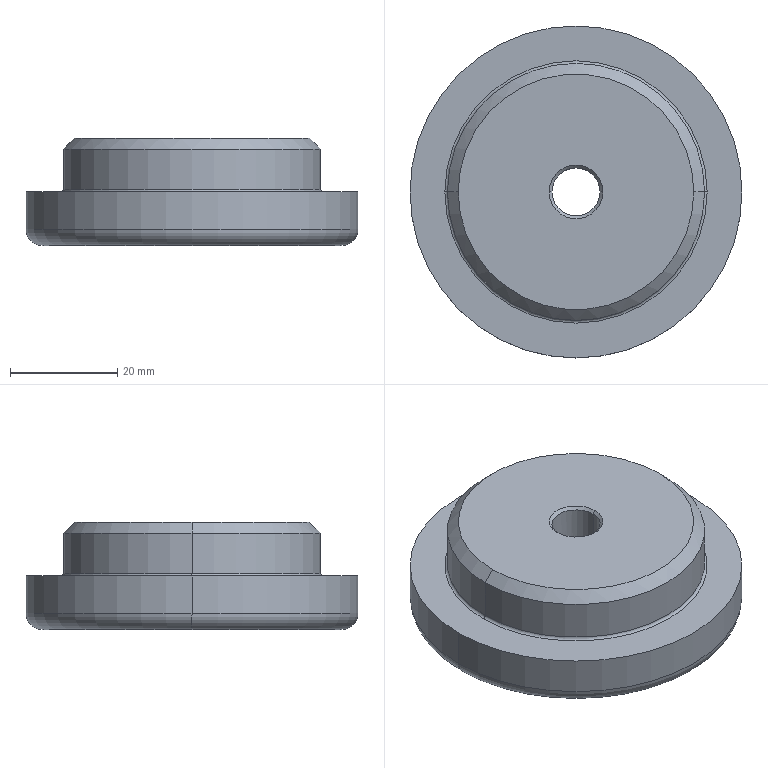Part | SolidWorks | features ICE 3, Fillet 2, 3DProfileFeature 1, Chamfer 1, Extrusion 1, HoleWzd 1 | 1 solid | 37 faces | box 62 x 62 x 20 mm | volume 45800 mm3 | plane 18 | cylinder 11 | torus 4 | cone 4 | commonest cylinder face diameters 6 x5 9 x2 48 x2 62 x2
STEP:
#1=CARTESIAN_POINT('',(-24.,0.,10.5));
#2=VERTEX_POINT('',#1);
#3=CARTESIAN_POINT('',(24.,0.,10.5));
#4=VERTEX_POINT('',#3);
#5=CARTESIAN_POINT('',(0.,0.,10.5));
#6=DIRECTION('',(0.,0.,1.));
#7=DIRECTION('',(1.,0.,0.));
#8=AXIS2_PLACEMENT_3D('',#5,#6,#7);
#9=CIRCLE('',#8,24.);
#10=EDGE_CURVE('',#2,#4,#9,.T.);
#11=ORIENTED_EDGE('',*,*,#10,.F.);
#12=CARTESIAN_POINT('',(-24.5,0.,10.));
#13=VERTEX_POINT('',#12);
#14=CARTESIAN_POINT('',(-24.5,0.,10.5));
#15=DIRECTION('',(0.,1.,0.));
#16=DIRECTION('',(-1.,0.,0.));
#17=AXIS2_PLACEMENT_3D('',#14,#15,#16);
#18=CIRCLE('',#17,0.5);
#19=EDGE_CURVE('',#2,#13,#18,.T.);
#20=ORIENTED_EDGE('',*,*,#19,.T.);
#21=CARTESIAN_POINT('',(24.5,0.,10.));
#22=VERTEX_POINT('',#21);
#23=CARTESIAN_POINT('',(0.,0.,10.));
#24=DIRECTION('',(0.,0.,-1.));
#25=DIRECTION('',(1.,0.,0.));
#26=AXIS2_PLACEMENT_3D('',#23,#24,#25);
#27=CIRCLE('',#26,24.5);
#28=EDGE_CURVE('',#22,#13,#27,.T.);
#29=ORIENTED_EDGE('',*,*,#28,.F.);
#30=CARTESIAN_POINT('',(24.5,0.,10.5));
#31=DIRECTION('',(0.,-1.,0.));
#32=DIRECTION('',(0.,0.,-1.));
#33=AXIS2_PLACEMENT_3D('',#30,#31,#32);
#34=CIRCLE('',#33,0.5);
#35=EDGE_CURVE('',#4,#22,#34,.T.);
#36=ORIENTED_EDGE('',*,*,#35,.F.);
#37=EDGE_LOOP('',(#11,#20,#29,#36));
#38=FACE_OUTER_BOUND('',#37,.T.);
#39=CARTESIAN_POINT('',(0.,0.,10.5));
#40=DIRECTION('',(0.,0.,1.));
#41=DIRECTION('',(1.,0.,0.));
#42=AXIS2_PLACEMENT_3D('',#39,#40,#41);
#43=TOROIDAL_SURFACE('',#42,24.5,0.5);
#44=ADVANCED_FACE('',(#38),#43,.F.);
#45=CARTESIAN_POINT('',(-28.,0.,1.));
#46=VERTEX_POINT('',#45);
#47=CARTESIAN_POINT('',(-25.,3.,1.));
#48=VERTEX_POINT('',#47);
#49=CARTESIAN_POINT('',(-25.,0.,1.));
#50=DIRECTION('',(0.,0.,-1.));
#51=DIRECTION('',(-1.,0.,0.));
#52=AXIS2_PLACEMENT_3D('',#49,#50,#51);
#53=CIRCLE('',#52,3.);
#54=EDGE_CURVE('',#46,#48,#53,.T.);
#55=ORIENTED_EDGE('',*,*,#54,.F.);
#56=CARTESIAN_POINT('',(-28.,0.,0.));
#57=VERTEX_POINT('',#56);
#58=CARTESIAN_POINT('',(-28.,0.,1.));
#59=DIRECTION('',(0.,0.,-1.));
#60=VECTOR('',#59,1000.);
#61=LINE('',#58,#60);
#62=EDGE_CURVE('',#46,#57,#61,.T.);
#63=ORIENTED_EDGE('',*,*,#62,.T.);
#64=CARTESIAN_POINT('',(-25.,3.,0.));
#65=VERTEX_POINT('',#64);
#66=CARTESIAN_POINT('',(-25.,0.,0.));
#67=DIRECTION('',(0.,0.,-1.));
#68=DIRECTION('',(-1.,0.,0.));
#69=AXIS2_PLACEMENT_3D('',#66,#67,#68);
#70=CIRCLE('',#69,3.);
#71=EDGE_CURVE('',#57,#65,#70,.T.);
#72=ORIENTED_EDGE('',*,*,#71,.T.);
#73=CARTESIAN_POINT('',(-25.,3.,1.));
#74=DIRECTION('',(0.,0.,-1.));
#75=VECTOR('',#74,1000.);
#76=LINE('',#73,#75);
#77=EDGE_CURVE('',#48,#65,#76,.T.);
#78=ORIENTED_EDGE('',*,*,#77,.F.);
#79=EDGE_LOOP('',(#55,#63,#72,#78));
#80=FACE_OUTER_BOUND('',#79,.T.);
#81=CARTESIAN_POINT('',(-25.,0.,1.));
#82=DIRECTION('',(0.,0.,-1.));
#83=DIRECTION('',(-1.,0.,0.));
#84=AXIS2_PLACEMENT_3D('',#81,#82,#83);
#85=CYLINDRICAL_SURFACE('',#84,3.);
#86=ADVANCED_FACE('',(#80),#85,.F.);
#87=CARTESIAN_POINT('',(-4.5,0.,19.475));
#88=VERTEX_POINT('',#87);
#89=CARTESIAN_POINT('',(4.5,0.,19.475));
#90=VERTEX_POINT('',#89);
#91=CARTESIAN_POINT('',(0.,0.,19.475));
#92=DIRECTION('',(0.,0.,1.));
#93=DIRECTION('',(1.,0.,0.));
#94=AXIS2_PLACEMENT_3D('',#91,#92,#93);
#95=CIRCLE('',#94,4.5);
#96=EDGE_CURVE('',#88,#90,#95,.T.);
#97=ORIENTED_EDGE('',*,*,#96,.F.);
#98=CARTESIAN_POINT('',(-5.025,0.,20.));
#99=VERTEX_POINT('',#98);
#100=CARTESIAN_POINT('',(-5.025,0.,20.));
#101=DIRECTION('',(-0.7071,0.,0.7071));
#102=VECTOR('',#101,1000.);
#103=LINE('',#100,#102);
#104=EDGE_CURVE('',#88,#99,#103,.T.);
#105=ORIENTED_EDGE('',*,*,#104,.T.);
#106=CARTESIAN_POINT('',(5.025,0.,20.));
#107=VERTEX_POINT('',#106);
#108=CARTESIAN_POINT('',(0.,0.,20.));
#109=DIRECTION('',(0.,0.,1.));
#110=DIRECTION('',(1.,0.,0.));
#111=AXIS2_PLACEMENT_3D('',#108,#109,#110);
#112=CIRCLE('',#111,5.025);
#113=EDGE_CURVE('',#99,#107,#112,.T.);
#114=ORIENTED_EDGE('',*,*,#113,.T.);
#115=CARTESIAN_POINT('',(5.025,0.,20.));
#116=DIRECTION('',(0.7071,0.,0.7071));
#117=VECTOR('',#116,1000.);
#118=LINE('',#115,#117);
#119=EDGE_CURVE('',#90,#107,#118,.T.);
#120=ORIENTED_EDGE('',*,*,#119,.F.);
#121=EDGE_LOOP('',(#97,#105,#114,#120));
#122=FACE_OUTER_BOUND('',#121,.T.);
#123=CARTESIAN_POINT('',(0.,0.,20.));
#124=DIRECTION('',(0.,0.,1.));
#125=DIRECTION('',(1.,0.,0.));
#126=AXIS2_PLACEMENT_3D('',#123,#124,#125);
#127=CONICAL_SURFACE('',#126,5.025,0.7854);
#128=ADVANCED_FACE('',(#122),#127,.F.);
#129=CARTESIAN_POINT('',(-4.5,0.,1.));
#130=VERTEX_POINT('',#129);
#131=CARTESIAN_POINT('',(-3.354,-3.,1.));
#132=VERTEX_POINT('',#131);
#133=CARTESIAN_POINT('',(0.,0.,1.));
#134=DIRECTION('',(0.,0.,1.));
#135=DIRECTION('',(-1.,0.,0.));
#136=AXIS2_PLACEMENT_3D('',#133,#134,#135);
#137=CIRCLE('',#136,4.5);
#138=EDGE_CURVE('',#130,#132,#137,.T.);
#139=ORIENTED_EDGE('',*,*,#138,.F.);
#140=CARTESIAN_POINT('',(-4.5,0.,20.));
#141=DIRECTION('',(0.,0.,1.));
#142=VECTOR('',#141,1000.);
#143=LINE('',#140,#142);
#144=EDGE_CURVE('',#130,#88,#143,.T.);
#145=ORIENTED_EDGE('',*,*,#144,.T.);
#146=ORIENTED_EDGE('',*,*,#96,.T.);
#147=CARTESIAN_POINT('',(4.5,0.,1.));
#148=VERTEX_POINT('',#147);
#149=CARTESIAN_POINT('',(4.5,0.,20.));
#150=DIRECTION('',(0.,0.,1.));
#151=VECTOR('',#150,1000.);
#152=LINE('',#149,#151);
#153=EDGE_CURVE('',#148,#90,#152,.T.);
#154=ORIENTED_EDGE('',*,*,#153,.F.);
#155=CARTESIAN_POINT('',(3.354,-3.,1.));
#156=VERTEX_POINT('',#155);
#157=CARTESIAN_POINT('',(0.,0.,1.));
#158=DIRECTION('',(0.,0.,1.));
#159=DIRECTION('',(-1.,0.,0.));
#160=AXIS2_PLACEMENT_3D('',#157,#158,#159);
#161=CIRCLE('',#160,4.5);
#162=EDGE_CURVE('',#156,#148,#161,.T.);
#163=ORIENTED_EDGE('',*,*,#162,.F.);
#164=CARTESIAN_POINT('',(3.354,-3.,0.));
#165=VERTEX_POINT('',#164);
#166=CARTESIAN_POINT('',(3.354,-3.,20.));
#167=DIRECTION('',(0.,0.,-1.));
#168=VECTOR('',#167,1000.);
#169=LINE('',#166,#168);
#170=EDGE_CURVE('',#156,#165,#169,.T.);
#171=ORIENTED_EDGE('',*,*,#170,.T.);
#172=CARTESIAN_POINT('',(3.,-3.354,0.));
#173=VERTEX_POINT('',#172);
#174=CARTESIAN_POINT('',(0.,0.,0.));
#175=DIRECTION('',(0.,0.,1.));
#176=DIRECTION('',(1.,0.,0.));
#177=AXIS2_PLACEMENT_3D('',#174,#175,#176);
#178=CIRCLE('',#177,4.5);
#179=EDGE_CURVE('',#173,#165,#178,.T.);
#180=ORIENTED_EDGE('',*,*,#179,.F.);
#181=CARTESIAN_POINT('',(3.,-3.354,1.));
#182=VERTEX_POINT('',#181);
#183=CARTESIAN_POINT('',(3.,-3.354,20.));
#184=DIRECTION('',(0.,0.,1.));
#185=VECTOR('',#184,1000.);
#186=LINE('',#183,#185);
#187=EDGE_CURVE('',#173,#182,#186,.T.);
#188=ORIENTED_EDGE('',*,*,#187,.T.);
#189=CARTESIAN_POINT('',(-3.,-3.354,1.));
#190=VERTEX_POINT('',#189);
#191=CARTESIAN_POINT('',(0.,0.,1.));
#192=DIRECTION('',(0.,0.,1.));
#193=DIRECTION('',(-1.,0.,0.));
#194=AXIS2_PLACEMENT_3D('',#191,#192,#193);
#195=CIRCLE('',#194,4.5);
#196=EDGE_CURVE('',#190,#182,#195,.T.);
#197=ORIENTED_EDGE('',*,*,#196,.F.);
#198=CARTESIAN_POINT('',(-3.,-3.354,0.));
#199=VERTEX_POINT('',#198);
#200=CARTESIAN_POINT('',(-3.,-3.354,20.));
#201=DIRECTION('',(0.,0.,-1.));
#202=VECTOR('',#201,1000.);
#203=LINE('',#200,#202);
#204=EDGE_CURVE('',#190,#199,#203,.T.);
#205=ORIENTED_EDGE('',*,*,#204,.T.);
#206=CARTESIAN_POINT('',(-3.354,-3.,0.));
#207=VERTEX_POINT('',#206);
#208=CARTESIAN_POINT('',(0.,0.,0.));
#209=DIRECTION('',(0.,0.,1.));
#210=DIRECTION('',(1.,0.,0.));
#211=AXIS2_PLACEMENT_3D('',#208,#209,#210);
#212=CIRCLE('',#211,4.5);
#213=EDGE_CURVE('',#207,#199,#212,.T.);
#214=ORIENTED_EDGE('',*,*,#213,.F.);
#215=CARTESIAN_POINT('',(-3.354,-3.,20.));
#216=DIRECTION('',(0.,0.,1.));
#217=VECTOR('',#216,1000.);
#218=LINE('',#215,#217);
#219=EDGE_CURVE('',#207,#132,#218,.T.);
#220=ORIENTED_EDGE('',*,*,#219,.T.);
#221=EDGE_LOOP('',(#139,#145,#146,#154,#163,#171,#180,#188,#197,#205,#214,#220));
#222=FACE_OUTER_BOUND('',#221,.T.);
#223=CARTESIAN_POINT('',(0.,0.,20.));
#224=DIRECTION('',(0.,0.,1.));
#225=DIRECTION('',(1.,0.,0.));
#226=AXIS2_PLACEMENT_3D('',#223,#224,#225);
#227=CYLINDRICAL_SURFACE('',#226,4.5);
#228=ADVANCED_FACE('',(#222),#227,.F.);
#229=CARTESIAN_POINT('',(0.,28.,0.));
#230=VERTEX_POINT('',#229);
#231=CARTESIAN_POINT('',(0.,0.,0.));
#232=DIRECTION('',(0.,0.,-1.));
#233=DIRECTION('',(1.,0.,0.));
#234=AXIS2_PLACEMENT_3D('',#231,#232,#233);
#235=CIRCLE('',#234,28.);
#236=EDGE_CURVE('',#57,#230,#235,.T.);
#237=ORIENTED_EDGE('',*,*,#236,.F.);
#238=CARTESIAN_POINT('',(-31.,0.,3.));
#239=VERTEX_POINT('',#238);
#240=CARTESIAN_POINT('',(-28.,0.,3.));
#241=DIRECTION('',(0.,1.,0.));
#242=DIRECTION('',(-1.,0.,0.));
#243=AXIS2_PLACEMENT_3D('',#240,#241,#242);
#244=CIRCLE('',#243,3.);
#245=EDGE_CURVE('',#57,#239,#244,.T.);
#246=ORIENTED_EDGE('',*,*,#245,.T.);
#247=CARTESIAN_POINT('',(31.,0.,3.));
#248=VERTEX_POINT('',#247);
#249=CARTESIAN_POINT('',(0.,0.,3.));
#250=DIRECTION('',(0.,0.,1.));
#251=DIRECTION('',(1.,0.,0.));
#252=AXIS2_PLACEMENT_3D('',#249,#250,#251);
#253=CIRCLE('',#252,31.);
#254=EDGE_CURVE('',#248,#239,#253,.T.);
#255=ORIENTED_EDGE('',*,*,#254,.F.);
#256=CARTESIAN_POINT('',(28.,0.,0.));
#257=VERTEX_POINT('',#256);
#258=CARTESIAN_POINT('',(28.,0.,3.));
#259=DIRECTION('',(0.,-1.,0.));
#260=DIRECTION('',(0.,0.,-1.));
#261=AXIS2_PLACEMENT_3D('',#258,#259,#260);
#262=CIRCLE('',#261,3.);
#263=EDGE_CURVE('',#257,#248,#262,.T.);
#264=ORIENTED_EDGE('',*,*,#263,.F.);
#265=CARTESIAN_POINT('',(0.,0.,0.));
#266=DIRECTION('',(0.,0.,-1.));
#267=DIRECTION('',(1.,0.,0.));
#268=AXIS2_PLACEMENT_3D('',#265,#266,#267);
#269=CIRCLE('',#268,28.);
#270=EDGE_CURVE('',#230,#257,#269,.T.);
#271=ORIENTED_EDGE('',*,*,#270,.F.);
#272=EDGE_LOOP('',(#237,#246,#255,#264,#271));
#273=FACE_OUTER_BOUND('',#272,.T.);
#274=CARTESIAN_POINT('',(0.,0.,3.));
#275=DIRECTION('',(0.,0.,1.));
#276=DIRECTION('',(1.,0.,0.));
#277=AXIS2_PLACEMENT_3D('',#274,#275,#276);
#278=TOROIDAL_SURFACE('',#277,28.,3.);
#279=ADVANCED_FACE('',(#273),#278,.T.);
#280=CARTESIAN_POINT('',(22.,0.,20.));
#281=VERTEX_POINT('',#280);
#282=CARTESIAN_POINT('',(-22.,0.,20.));
#283=VERTEX_POINT('',#282);
#284=CARTESIAN_POINT('',(0.,0.,20.));
#285=DIRECTION('',(0.,0.,1.));
#286=DIRECTION('',(1.,0.,0.));
#287=AXIS2_PLACEMENT_3D('',#284,#285,#286);
#288=CIRCLE('',#287,22.);
#289=EDGE_CURVE('',#281,#283,#288,.T.);
#290=ORIENTED_EDGE('',*,*,#289,.F.);
#291=CARTESIAN_POINT('',(24.,0.,18.));
#292=VERTEX_POINT('',#291);
#293=CARTESIAN_POINT('',(22.,0.,20.));
#294=DIRECTION('',(0.7071,0.,-0.7071));
#295=VECTOR('',#294,1000.);
#296=LINE('',#293,#295);
#297=EDGE_CURVE('',#281,#292,#296,.T.);
#298=ORIENTED_EDGE('',*,*,#297,.T.);
#299=CARTESIAN_POINT('',(-24.,0.,18.));
#300=VERTEX_POINT('',#299);
#301=CARTESIAN_POINT('',(0.,0.,18.));
#302=DIRECTION('',(0.,0.,-1.));
#303=DIRECTION('',(1.,0.,0.));
#304=AXIS2_PLACEMENT_3D('',#301,#302,#303);
#305=CIRCLE('',#304,24.);
#306=EDGE_CURVE('',#300,#292,#305,.T.);
#307=ORIENTED_EDGE('',*,*,#306,.F.);
#308=CARTESIAN_POINT('',(-22.,0.,20.));
#309=DIRECTION('',(-0.7071,0.,-0.7071));
#310=VECTOR('',#309,1000.);
#311=LINE('',#308,#310);
#312=EDGE_CURVE('',#283,#300,#311,.T.);
#313=ORIENTED_EDGE('',*,*,#312,.F.);
#314=EDGE_LOOP('',(#290,#298,#307,#313));
#315=FACE_OUTER_BOUND('',#314,.T.);
#316=CARTESIAN_POINT('',(0.,0.,20.));
#317=DIRECTION('',(0.,0.,-1.));
#318=DIRECTION('',(-1.,0.,0.));
#319=AXIS2_PLACEMENT_3D('',#316,#317,#318);
#320=CONICAL_SURFACE('',#319,22.,0.7854);
#321=ADVANCED_FACE('',(#315),#320,.T.);
#322=ORIENTED_EDGE('',*,*,#306,.T.);
#323=CARTESIAN_POINT('',(24.,0.,20.));
#324=DIRECTION('',(0.,0.,-1.));
#325=VECTOR('',#324,1000.);
#326=LINE('',#323,#325);
#327=EDGE_CURVE('',#292,#4,#326,.T.);
#328=ORIENTED_EDGE('',*,*,#327,.T.);
#329=CARTESIAN_POINT('',(0.,0.,10.5));
#330=DIRECTION('',(0.,0.,1.));
#331=DIRECTION('',(1.,0.,0.));
#332=AXIS2_PLACEMENT_3D('',#329,#330,#331);
#333=CIRCLE('',#332,24.);
#334=EDGE_CURVE('',#4,#2,#333,.T.);
#335=ORIENTED_EDGE('',*,*,#334,.T.);
#336=CARTESIAN_POINT('',(-24.,0.,20.));
#337=DIRECTION('',(0.,0.,-1.));
#338=VECTOR('',#337,1000.);
#339=LINE('',#336,#338);
#340=EDGE_CURVE('',#300,#2,#339,.T.);
#341=ORIENTED_EDGE('',*,*,#340,.F.);
#342=EDGE_LOOP('',(#322,#328,#335,#341));
#343=FACE_OUTER_BOUND('',#342,.T.);
#344=CARTESIAN_POINT('',(0.,0.,20.));
#345=DIRECTION('',(0.,0.,-1.));
#346=DIRECTION('',(-1.,0.,0.));
#347=AXIS2_PLACEMENT_3D('',#344,#345,#346);
#348=CYLINDRICAL_SURFACE('',#347,24.);
#349=ADVANCED_FACE('',(#343),#348,.T.);
#350=CARTESIAN_POINT('',(31.,0.,10.));
#351=VERTEX_POINT('',#350);
#352=CARTESIAN_POINT('',(-31.,0.,10.));
#353=VERTEX_POINT('',#352);
#354=CARTESIAN_POINT('',(0.,0.,10.));
#355=DIRECTION('',(0.,0.,1.));
#356=DIRECTION('',(1.,0.,0.));
#357=AXIS2_PLACEMENT_3D('',#354,#355,#356);
#358=CIRCLE('',#357,31.);
#359=EDGE_CURVE('',#351,#353,#358,.T.);
#360=ORIENTED_EDGE('',*,*,#359,.F.);
#361=CARTESIAN_POINT('',(31.,0.,10.));
#362=DIRECTION('',(0.,0.,-1.));
#363=VECTOR('',#362,1000.);
#364=LINE('',#361,#363);
#365=EDGE_CURVE('',#351,#248,#364,.T.);
#366=ORIENTED_EDGE('',*,*,#365,.T.);
#367=ORIENTED_EDGE('',*,*,#254,.T.);
#368=CARTESIAN_POINT('',(-31.,0.,10.));
#369=DIRECTION('',(0.,0.,-1.));
#370=VECTOR('',#369,1000.);
#371=LINE('',#368,#370);
#372=EDGE_CURVE('',#353,#239,#371,.T.);
#373=ORIENTED_EDGE('',*,*,#372,.F.);
#374=EDGE_LOOP('',(#360,#366,#367,#373));
#375=FACE_OUTER_BOUND('',#374,.T.);
#376=CARTESIAN_POINT('',(0.,0.,10.));
#377=DIRECTION('',(0.,0.,-1.));
#378=DIRECTION('',(-1.,0.,0.));
#379=AXIS2_PLACEMENT_3D('',#376,#377,#378);
#380=CYLINDRICAL_SURFACE('',#379,31.);
#381=ADVANCED_FACE('',(#375),#380,.T.);
#382=CARTESIAN_POINT('',(25.,3.,0.));
#383=VERTEX_POINT('',#382);
#384=CARTESIAN_POINT('',(25.,0.,0.));
#385=DIRECTION('',(0.,0.,-1.));
#386=DIRECTION('',(-1.,0.,0.));
#387=AXIS2_PLACEMENT_3D('',#384,#385,#386);
#388=CIRCLE('',#387,3.);
#389=EDGE_CURVE('',#383,#257,#388,.T.);
#390=ORIENTED_EDGE('',*,*,#389,.F.);
#391=CARTESIAN_POINT('',(3.354,3.,0.));
#392=VERTEX_POINT('',#391);
#393=CARTESIAN_POINT('',(25.,3.,0.));
#394=DIRECTION('',(1.,0.,0.));
#395=VECTOR('',#394,1000.);
#396=LINE('',#393,#395);
#397=EDGE_CURVE('',#392,#383,#396,.T.);
#398=ORIENTED_EDGE('',*,*,#397,.F.);
#399=CARTESIAN_POINT('',(3.,3.354,0.));
#400=VERTEX_POINT('',#399);
#401=CARTESIAN_POINT('',(0.,0.,0.));
#402=DIRECTION('',(0.,0.,1.));
#403=DIRECTION('',(1.,0.,0.));
#404=AXIS2_PLACEMENT_3D('',#401,#402,#403);
#405=CIRCLE('',#404,4.5);
#406=EDGE_CURVE('',#392,#400,#405,.T.);
#407=ORIENTED_EDGE('',*,*,#406,.T.);
#408=CARTESIAN_POINT('',(3.,25.,0.));
#409=VERTEX_POINT('',#408);
#410=CARTESIAN_POINT('',(3.,-25.,0.));
#411=DIRECTION('',(0.,-1.,0.));
#412=VECTOR('',#411,1000.);
#413=LINE('',#410,#412);
#414=EDGE_CURVE('',#409,#400,#413,.T.);
#415=ORIENTED_EDGE('',*,*,#414,.F.);
#416=CARTESIAN_POINT('',(0.,25.,0.));
#417=DIRECTION('',(0.,0.,-1.));
#418=DIRECTION('',(-1.,0.,0.));
#419=AXIS2_PLACEMENT_3D('',#416,#417,#418);
#420=CIRCLE('',#419,3.);
#421=EDGE_CURVE('',#230,#409,#420,.T.);
#422=ORIENTED_EDGE('',*,*,#421,.F.);
#423=ORIENTED_EDGE('',*,*,#270,.T.);
#424=EDGE_LOOP('',(#390,#398,#407,#415,#422,#423));
#425=FACE_OUTER_BOUND('',#424,.T.);
#426=CARTESIAN_POINT('',(0.,0.,0.));
#427=DIRECTION('',(0.,0.,1.));
#428=DIRECTION('',(1.,0.,0.));
#429=AXIS2_PLACEMENT_3D('',#426,#427,#428);
#430=PLANE('',#429);
#431=ADVANCED_FACE('',(#425),#430,.F.);
#432=CARTESIAN_POINT('',(-3.,3.354,0.));
#433=VERTEX_POINT('',#432);
#434=CARTESIAN_POINT('',(-3.354,3.,0.));
#435=VERTEX_POINT('',#434);
#436=CARTESIAN_POINT('',(0.,0.,0.));
#437=DIRECTION('',(0.,0.,1.));
#438=DIRECTION('',(1.,0.,0.));
#439=AXIS2_PLACEMENT_3D('',#436,#437,#438);
#440=CIRCLE('',#439,4.5);
#441=EDGE_CURVE('',#433,#435,#440,.T.);
#442=ORIENTED_EDGE('',*,*,#441,.T.);
#443=CARTESIAN_POINT('',(25.,3.,0.));
#444=DIRECTION('',(1.,0.,0.));
#445=VECTOR('',#444,1000.);
#446=LINE('',#443,#445);
#447=EDGE_CURVE('',#65,#435,#446,.T.);
#448=ORIENTED_EDGE('',*,*,#447,.F.);
#449=ORIENTED_EDGE('',*,*,#71,.F.);
#450=ORIENTED_EDGE('',*,*,#236,.T.);
#451=CARTESIAN_POINT('',(-3.,25.,0.));
#452=VERTEX_POINT('',#451);
#453=CARTESIAN_POINT('',(0.,25.,0.));
#454=DIRECTION('',(0.,0.,-1.));
#455=DIRECTION('',(-1.,0.,0.));
#456=AXIS2_PLACEMENT_3D('',#453,#454,#455);
#457=CIRCLE('',#456,3.);
#458=EDGE_CURVE('',#452,#230,#457,.T.);
#459=ORIENTED_EDGE('',*,*,#458,.F.);
#460=CARTESIAN_POINT('',(-3.,-25.,0.));
#461=DIRECTION('',(0.,1.,0.));
#462=VECTOR('',#461,1000.);
#463=LINE('',#460,#462);
#464=EDGE_CURVE('',#433,#452,#463,.T.);
#465=ORIENTED_EDGE('',*,*,#464,.F.);
#466=EDGE_LOOP('',(#442,#448,#449,#450,#459,#465));
#467=FACE_OUTER_BOUND('',#466,.T.);
#468=CARTESIAN_POINT('',(0.,0.,0.));
#469=DIRECTION('',(0.,0.,1.));
#470=DIRECTION('',(1.,0.,0.));
#471=AXIS2_PLACEMENT_3D('',#468,#469,#470);
#472=PLANE('',#471);
#473=ADVANCED_FACE('',(#467),#472,.F.);
#474=CARTESIAN_POINT('',(25.,-3.,0.));
#475=VERTEX_POINT('',#474);
#476=CARTESIAN_POINT('',(25.,-3.,0.));
#477=DIRECTION('',(-1.,0.,0.));
#478=VECTOR('',#477,1000.);
#479=LINE('',#476,#478);
#480=EDGE_CURVE('',#475,#165,#479,.T.);
#481=ORIENTED_EDGE('',*,*,#480,.F.);
#482=CARTESIAN_POINT('',(25.,0.,0.));
#483=DIRECTION('',(0.,0.,-1.));
#484=DIRECTION('',(-1.,0.,0.));
#485=AXIS2_PLACEMENT_3D('',#482,#483,#484);
#486=CIRCLE('',#485,3.);
#487=EDGE_CURVE('',#257,#475,#486,.T.);
#488=ORIENTED_EDGE('',*,*,#487,.F.);
#489=CARTESIAN_POINT('',(0.,-28.,0.));
#490=VERTEX_POINT('',#489);
#491=CARTESIAN_POINT('',(0.,0.,0.));
#492=DIRECTION('',(0.,0.,-1.));
#493=DIRECTION('',(1.,0.,0.));
#494=AXIS2_PLACEMENT_3D('',#491,#492,#493);
#495=CIRCLE('',#494,28.);
#496=EDGE_CURVE('',#257,#490,#495,.T.);
#497=ORIENTED_EDGE('',*,*,#496,.T.);
#498=CARTESIAN_POINT('',(3.,-25.,0.));
#499=VERTEX_POINT('',#498);
#500=CARTESIAN_POINT('',(0.,-25.,0.));
#501=DIRECTION('',(0.,0.,-1.));
#502=DIRECTION('',(-1.,0.,0.));
#503=AXIS2_PLACEMENT_3D('',#500,#501,#502);
#504=CIRCLE('',#503,3.);
#505=EDGE_CURVE('',#499,#490,#504,.T.);
#506=ORIENTED_EDGE('',*,*,#505,.F.);
#507=CARTESIAN_POINT('',(3.,-25.,0.));
#508=DIRECTION('',(0.,-1.,0.));
#509=VECTOR('',#508,1000.);
#510=LINE('',#507,#509);
#511=EDGE_CURVE('',#173,#499,#510,.T.);
#512=ORIENTED_EDGE('',*,*,#511,.F.);
#513=ORIENTED_EDGE('',*,*,#179,.T.);
#514=EDGE_LOOP('',(#481,#488,#497,#506,#512,#513));
#515=FACE_OUTER_BOUND('',#514,.T.);
#516=CARTESIAN_POINT('',(0.,0.,0.));
#517=DIRECTION('',(0.,0.,1.));
#518=DIRECTION('',(1.,0.,0.));
#519=AXIS2_PLACEMENT_3D('',#516,#517,#518);
#520=PLANE('',#519);
#521=ADVANCED_FACE('',(#515),#520,.F.);
#522=ORIENTED_EDGE('',*,*,#365,.F.);
#523=CARTESIAN_POINT('',(0.,0.,10.));
#524=DIRECTION('',(0.,0.,1.));
#525=DIRECTION('',(1.,0.,0.));
#526=AXIS2_PLACEMENT_3D('',#523,#524,#525);
#527=CIRCLE('',#526,31.);
#528=EDGE_CURVE('',#353,#351,#527,.T.);
#529=ORIENTED_EDGE('',*,*,#528,.F.);
#530=ORIENTED_EDGE('',*,*,#372,.T.);
#531=CARTESIAN_POINT('',(0.,0.,3.));
#532=DIRECTION('',(0.,0.,1.));
#533=DIRECTION('',(1.,0.,0.));
#534=AXIS2_PLACEMENT_3D('',#531,#532,#533);
#535=CIRCLE('',#534,31.);
#536=EDGE_CURVE('',#239,#248,#535,.T.);
#537=ORIENTED_EDGE('',*,*,#536,.T.);
#538=EDGE_LOOP('',(#522,#529,#530,#537));
#539=FACE_OUTER_BOUND('',#538,.T.);
#540=CARTESIAN_POINT('',(0.,0.,10.));
#541=DIRECTION('',(0.,0.,-1.));
#542=DIRECTION('',(-1.,0.,0.));
#543=AXIS2_PLACEMENT_3D('',#540,#541,#542);
#544=CYLINDRICAL_SURFACE('',#543,31.);
#545=ADVANCED_FACE('',(#539),#544,.T.);
#546=ORIENTED_EDGE('',*,*,#28,.T.);
#547=CARTESIAN_POINT('',(0.,0.,10.));
#548=DIRECTION('',(0.,0.,-1.));
#549=DIRECTION('',(1.,0.,0.));
#550=AXIS2_PLACEMENT_3D('',#547,#548,#549);
#551=CIRCLE('',#550,24.5);
#552=EDGE_CURVE('',#13,#22,#551,.T.);
#553=ORIENTED_EDGE('',*,*,#552,.T.);
#554=EDGE_LOOP('',(#546,#553));
#555=FACE_BOUND('',#554,.T.);
#556=ORIENTED_EDGE('',*,*,#528,.T.);
#557=ORIENTED_EDGE('',*,*,#359,.T.);
#558=EDGE_LOOP('',(#556,#557));
#559=FACE_OUTER_BOUND('',#558,.T.);
#560=CARTESIAN_POINT('',(0.,0.,10.));
#561=DIRECTION('',(0.,0.,1.));
#562=DIRECTION('',(1.,0.,0.));
#563=AXIS2_PLACEMENT_3D('',#560,#561,#562);
#564=PLANE('',#563);
#565=ADVANCED_FACE('',(#555,#559),#564,.T.);
#566=CARTESIAN_POINT('',(0.,0.,0.));
#567=DIRECTION('',(0.,0.,-1.));
#568=DIRECTION('',(1.,0.,0.));
#569=AXIS2_PLACEMENT_3D('',#566,#567,#568);
#570=CIRCLE('',#569,28.);
#571=EDGE_CURVE('',#490,#57,#570,.T.);
#572=ORIENTED_EDGE('',*,*,#571,.T.);
#573=CARTESIAN_POINT('',(-25.,-3.,0.));
#574=VERTEX_POINT('',#573);
#575=CARTESIAN_POINT('',(-25.,0.,0.));
#576=DIRECTION('',(0.,0.,-1.));
#577=DIRECTION('',(-1.,0.,0.));
#578=AXIS2_PLACEMENT_3D('',#575,#576,#577);
#579=CIRCLE('',#578,3.);
#580=EDGE_CURVE('',#574,#57,#579,.T.);
#581=ORIENTED_EDGE('',*,*,#580,.F.);
#582=CARTESIAN_POINT('',(25.,-3.,0.));
#583=DIRECTION('',(-1.,0.,0.));
#584=VECTOR('',#583,1000.);
#585=LINE('',#582,#584);
#586=EDGE_CURVE('',#207,#574,#585,.T.);
#587=ORIENTED_EDGE('',*,*,#586,.F.);
#588=ORIENTED_EDGE('',*,*,#213,.T.);
#589=CARTESIAN_POINT('',(-3.,-25.,0.));
#590=VERTEX_POINT('',#589);
#591=CARTESIAN_POINT('',(-3.,-25.,0.));
#592=DIRECTION('',(0.,1.,0.));
#593=VECTOR('',#592,1000.);
#594=LINE('',#591,#593);
#595=EDGE_CURVE('',#590,#199,#594,.T.);
#596=ORIENTED_EDGE('',*,*,#595,.F.);
#597=CARTESIAN_POINT('',(0.,-25.,0.));
#598=DIRECTION('',(0.,0.,-1.));
#599=DIRECTION('',(-1.,0.,0.));
#600=AXIS2_PLACEMENT_3D('',#597,#598,#599);
#601=CIRCLE('',#600,3.);
#602=EDGE_CURVE('',#490,#590,#601,.T.);
#603=ORIENTED_EDGE('',*,*,#602,.F.);
#604=EDGE_LOOP('',(#572,#581,#587,#588,#596,#603));
#605=FACE_OUTER_BOUND('',#604,.T.);
#606=CARTESIAN_POINT('',(0.,0.,0.));
#607=DIRECTION('',(0.,0.,1.));
#608=DIRECTION('',(1.,0.,0.));
#609=AXIS2_PLACEMENT_3D('',#606,#607,#608);
#610=PLANE('',#609);
#611=ADVANCED_FACE('',(#605),#610,.F.);
#612=ORIENTED_EDGE('',*,*,#327,.F.);
#613=CARTESIAN_POINT('',(0.,0.,18.));
#614=DIRECTION('',(0.,0.,-1.));
#615=DIRECTION('',(1.,0.,0.));
#616=AXIS2_PLACEMENT_3D('',#613,#614,#615);
#617=CIRCLE('',#616,24.);
#618=EDGE_CURVE('',#292,#300,#617,.T.);
#619=ORIENTED_EDGE('',*,*,#618,.T.);
#620=ORIENTED_EDGE('',*,*,#340,.T.);
#621=ORIENTED_EDGE('',*,*,#10,.T.);
#622=EDGE_LOOP('',(#612,#619,#620,#621));
#623=FACE_OUTER_BOUND('',#622,.T.);
#624=CARTESIAN_POINT('',(0.,0.,20.));
#625=DIRECTION('',(0.,0.,-1.));
#626=DIRECTION('',(-1.,0.,0.));
#627=AXIS2_PLACEMENT_3D('',#624,#625,#626);
#628=CYLINDRICAL_SURFACE('',#627,24.);
#629=ADVANCED_FACE('',(#623),#628,.T.);
#630=CARTESIAN_POINT('',(0.,0.,20.));
#631=DIRECTION('',(0.,0.,1.));
#632=DIRECTION('',(1.,0.,0.));
#633=AXIS2_PLACEMENT_3D('',#630,#631,#632);
#634=CIRCLE('',#633,5.025);
#635=EDGE_CURVE('',#107,#99,#634,.T.);
#636=ORIENTED_EDGE('',*,*,#635,.F.);
#637=ORIENTED_EDGE('',*,*,#113,.F.);
#638=EDGE_LOOP('',(#636,#637));
#639=FACE_BOUND('',#638,.T.);
#640=CARTESIAN_POINT('',(0.,0.,20.));
#641=DIRECTION('',(0.,0.,1.));
#642=DIRECTION('',(1.,0.,0.));
#643=AXIS2_PLACEMENT_3D('',#640,#641,#642);
#644=CIRCLE('',#643,22.);
#645=EDGE_CURVE('',#283,#281,#644,.T.);
#646=ORIENTED_EDGE('',*,*,#645,.T.);
#647=ORIENTED_EDGE('',*,*,#289,.T.);
#648=EDGE_LOOP('',(#646,#647));
#649=FACE_OUTER_BOUND('',#648,.T.);
#650=CARTESIAN_POINT('',(0.,0.,20.));
#651=DIRECTION('',(0.,0.,1.));
#652=DIRECTION('',(1.,0.,0.));
#653=AXIS2_PLACEMENT_3D('',#650,#651,#652);
#654=PLANE('',#653);
#655=ADVANCED_FACE('',(#639,#649),#654,.T.);
#656=ORIENTED_EDGE('',*,*,#297,.F.);
#657=ORIENTED_EDGE('',*,*,#645,.F.);
#658=ORIENTED_EDGE('',*,*,#312,.T.);
#659=ORIENTED_EDGE('',*,*,#618,.F.);
#660=EDGE_LOOP('',(#656,#657,#658,#659));
#661=FACE_OUTER_BOUND('',#660,.T.);
#662=CARTESIAN_POINT('',(0.,0.,20.));
#663=DIRECTION('',(0.,0.,-1.));
#664=DIRECTION('',(-1.,0.,0.));
#665=AXIS2_PLACEMENT_3D('',#662,#663,#664);
#666=CONICAL_SURFACE('',#665,22.,0.7854);
#667=ADVANCED_FACE('',(#661),#666,.T.);
#668=ORIENTED_EDGE('',*,*,#245,.F.);
#669=ORIENTED_EDGE('',*,*,#571,.F.);
#670=ORIENTED_EDGE('',*,*,#496,.F.);
#671=ORIENTED_EDGE('',*,*,#263,.T.);
#672=ORIENTED_EDGE('',*,*,#536,.F.);
#673=EDGE_LOOP('',(#668,#669,#670,#671,#672));
#674=FACE_OUTER_BOUND('',#673,.T.);
#675=CARTESIAN_POINT('',(0.,0.,3.));
#676=DIRECTION('',(0.,0.,1.));
#677=DIRECTION('',(1.,0.,0.));
#678=AXIS2_PLACEMENT_3D('',#675,#676,#677);
#679=TOROIDAL_SURFACE('',#678,28.,3.);
#680=ADVANCED_FACE('',(#674),#679,.T.);
#681=ORIENTED_EDGE('',*,*,#144,.F.);
#682=CARTESIAN_POINT('',(-3.354,3.,1.));
#683=VERTEX_POINT('',#682);
#684=CARTESIAN_POINT('',(0.,0.,1.));
#685=DIRECTION('',(0.,0.,1.));
#686=DIRECTION('',(-1.,0.,0.));
#687=AXIS2_PLACEMENT_3D('',#684,#685,#686);
#688=CIRCLE('',#687,4.5);
#689=EDGE_CURVE('',#683,#130,#688,.T.);
#690=ORIENTED_EDGE('',*,*,#689,.F.);
#691=CARTESIAN_POINT('',(-3.354,3.,20.));
#692=DIRECTION('',(0.,0.,-1.));
#693=VECTOR('',#692,1000.);
#694=LINE('',#691,#693);
#695=EDGE_CURVE('',#683,#435,#694,.T.);
#696=ORIENTED_EDGE('',*,*,#695,.T.);
#697=ORIENTED_EDGE('',*,*,#441,.F.);
#698=CARTESIAN_POINT('',(-3.,3.354,1.));
#699=VERTEX_POINT('',#698);
#700=CARTESIAN_POINT('',(-3.,3.354,20.));
#701=DIRECTION('',(0.,0.,1.));
#702=VECTOR('',#701,1000.);
#703=LINE('',#700,#702);
#704=EDGE_CURVE('',#433,#699,#703,.T.);
#705=ORIENTED_EDGE('',*,*,#704,.T.);
#706=CARTESIAN_POINT('',(3.,3.354,1.));
#707=VERTEX_POINT('',#706);
#708=CARTESIAN_POINT('',(0.,0.,1.));
#709=DIRECTION('',(0.,0.,1.));
#710=DIRECTION('',(-1.,0.,0.));
#711=AXIS2_PLACEMENT_3D('',#708,#709,#710);
#712=CIRCLE('',#711,4.5);
#713=EDGE_CURVE('',#707,#699,#712,.T.);
#714=ORIENTED_EDGE('',*,*,#713,.F.);
#715=CARTESIAN_POINT('',(3.,3.354,20.));
#716=DIRECTION('',(0.,0.,-1.));
#717=VECTOR('',#716,1000.);
#718=LINE('',#715,#717);
#719=EDGE_CURVE('',#707,#400,#718,.T.);
#720=ORIENTED_EDGE('',*,*,#719,.T.);
#721=ORIENTED_EDGE('',*,*,#406,.F.);
#722=CARTESIAN_POINT('',(3.354,3.,1.));
#723=VERTEX_POINT('',#722);
#724=CARTESIAN_POINT('',(3.354,3.,20.));
#725=DIRECTION('',(0.,0.,1.));
#726=VECTOR('',#725,1000.);
#727=LINE('',#724,#726);
#728=EDGE_CURVE('',#392,#723,#727,.T.);
#729=ORIENTED_EDGE('',*,*,#728,.T.);
#730=CARTESIAN_POINT('',(0.,0.,1.));
#731=DIRECTION('',(0.,0.,1.));
#732=DIRECTION('',(-1.,0.,0.));
#733=AXIS2_PLACEMENT_3D('',#730,#731,#732);
#734=CIRCLE('',#733,4.5);
#735=EDGE_CURVE('',#148,#723,#734,.T.);
#736=ORIENTED_EDGE('',*,*,#735,.F.);
#737=ORIENTED_EDGE('',*,*,#153,.T.);
#738=CARTESIAN_POINT('',(0.,0.,19.475));
#739=DIRECTION('',(0.,0.,1.));
#740=DIRECTION('',(1.,0.,0.));
#741=AXIS2_PLACEMENT_3D('',#738,#739,#740);
#742=CIRCLE('',#741,4.5);
#743=EDGE_CURVE('',#90,#88,#742,.T.);
#744=ORIENTED_EDGE('',*,*,#743,.T.);
#745=EDGE_LOOP('',(#681,#690,#696,#697,#705,#714,#720,#721,#729,#736,#737,#744));
#746=FACE_OUTER_BOUND('',#745,.T.);
#747=CARTESIAN_POINT('',(0.,0.,20.));
#748=DIRECTION('',(0.,0.,1.));
#749=DIRECTION('',(1.,0.,0.));
#750=AXIS2_PLACEMENT_3D('',#747,#748,#749);
#751=CYLINDRICAL_SURFACE('',#750,4.5);
#752=ADVANCED_FACE('',(#746),#751,.F.);
#753=ORIENTED_EDGE('',*,*,#104,.F.);
#754=ORIENTED_EDGE('',*,*,#743,.F.);
#755=ORIENTED_EDGE('',*,*,#119,.T.);
#756=ORIENTED_EDGE('',*,*,#635,.T.);
#757=EDGE_LOOP('',(#753,#754,#755,#756));
#758=FACE_OUTER_BOUND('',#757,.T.);
#759=CARTESIAN_POINT('',(0.,0.,20.));
#760=DIRECTION('',(0.,0.,1.));
#761=DIRECTION('',(1.,0.,0.));
#762=AXIS2_PLACEMENT_3D('',#759,#760,#761);
#763=CONICAL_SURFACE('',#762,5.025,0.7854);
#764=ADVANCED_FACE('',(#758),#763,.F.);
#765=ORIENTED_EDGE('',*,*,#713,.T.);
#766=CARTESIAN_POINT('',(-3.,25.,1.));
#767=VERTEX_POINT('',#766);
#768=CARTESIAN_POINT('',(-3.,-25.,1.));
#769=DIRECTION('',(0.,1.,0.));
#770=VECTOR('',#769,1000.);
#771=LINE('',#768,#770);
#772=EDGE_CURVE('',#699,#767,#771,.T.);
#773=ORIENTED_EDGE('',*,*,#772,.T.);
#774=CARTESIAN_POINT('',(3.,25.,1.));
#775=VERTEX_POINT('',#774);
#776=CARTESIAN_POINT('',(0.,25.,1.));
#777=DIRECTION('',(0.,0.,-1.));
#778=DIRECTION('',(-1.,0.,0.));
#779=AXIS2_PLACEMENT_3D('',#776,#777,#778);
#780=CIRCLE('',#779,3.);
#781=EDGE_CURVE('',#767,#775,#780,.T.);
#782=ORIENTED_EDGE('',*,*,#781,.T.);
#783=CARTESIAN_POINT('',(3.,-25.,1.));
#784=DIRECTION('',(0.,-1.,0.));
#785=VECTOR('',#784,1000.);
#786=LINE('',#783,#785);
#787=EDGE_CURVE('',#775,#707,#786,.T.);
#788=ORIENTED_EDGE('',*,*,#787,.T.);
#789=EDGE_LOOP('',(#765,#773,#782,#788));
#790=FACE_OUTER_BOUND('',#789,.T.);
#791=CARTESIAN_POINT('',(0.,-25.,1.));
#792=DIRECTION('',(0.,0.,-1.));
#793=DIRECTION('',(-1.,0.,0.));
#794=AXIS2_PLACEMENT_3D('',#791,#792,#793);
#795=PLANE('',#794);
#796=ADVANCED_FACE('',(#790),#795,.T.);
#797=ORIENTED_EDGE('',*,*,#464,.T.);
#798=CARTESIAN_POINT('',(-3.,25.,1.));
#799=DIRECTION('',(0.,0.,-1.));
#800=VECTOR('',#799,1000.);
#801=LINE('',#798,#800);
#802=EDGE_CURVE('',#767,#452,#801,.T.);
#803=ORIENTED_EDGE('',*,*,#802,.F.);
#804=ORIENTED_EDGE('',*,*,#772,.F.);
#805=ORIENTED_EDGE('',*,*,#704,.F.);
#806=EDGE_LOOP('',(#797,#803,#804,#805));
#807=FACE_OUTER_BOUND('',#806,.T.);
#808=CARTESIAN_POINT('',(-3.,-25.,1.));
#809=DIRECTION('',(-1.,0.,0.));
#810=DIRECTION('',(0.,-1.,0.));
#811=AXIS2_PLACEMENT_3D('',#808,#809,#810);
#812=PLANE('',#811);
#813=ADVANCED_FACE('',(#807),#812,.F.);
#814=ORIENTED_EDGE('',*,*,#787,.F.);
#815=CARTESIAN_POINT('',(3.,25.,1.));
#816=DIRECTION('',(0.,0.,-1.));
#817=VECTOR('',#816,1000.);
#818=LINE('',#815,#817);
#819=EDGE_CURVE('',#775,#409,#818,.T.);
#820=ORIENTED_EDGE('',*,*,#819,.T.);
#821=ORIENTED_EDGE('',*,*,#414,.T.);
#822=ORIENTED_EDGE('',*,*,#719,.F.);
#823=EDGE_LOOP('',(#814,#820,#821,#822));
#824=FACE_OUTER_BOUND('',#823,.T.);
#825=CARTESIAN_POINT('',(3.,-25.,1.));
#826=DIRECTION('',(1.,0.,0.));
#827=DIRECTION('',(0.,1.,0.));
#828=AXIS2_PLACEMENT_3D('',#825,#826,#827);
#829=PLANE('',#828);
#830=ADVANCED_FACE('',(#824),#829,.F.);
#831=ORIENTED_EDGE('',*,*,#458,.T.);
#832=ORIENTED_EDGE('',*,*,#421,.T.);
#833=ORIENTED_EDGE('',*,*,#819,.F.);
#834=ORIENTED_EDGE('',*,*,#781,.F.);
#835=ORIENTED_EDGE('',*,*,#802,.T.);
#836=EDGE_LOOP('',(#831,#832,#833,#834,#835));
#837=FACE_OUTER_BOUND('',#836,.T.);
#838=CARTESIAN_POINT('',(0.,25.,1.));
#839=DIRECTION('',(0.,0.,-1.));
#840=DIRECTION('',(-1.,0.,0.));
#841=AXIS2_PLACEMENT_3D('',#838,#839,#840);
#842=CYLINDRICAL_SURFACE('',#841,3.);
#843=ADVANCED_FACE('',(#837),#842,.F.);
#844=ORIENTED_EDGE('',*,*,#511,.T.);
#845=CARTESIAN_POINT('',(3.,-25.,1.));
#846=VERTEX_POINT('',#845);
#847=CARTESIAN_POINT('',(3.,-25.,1.));
#848=DIRECTION('',(0.,0.,-1.));
#849=VECTOR('',#848,1000.);
#850=LINE('',#847,#849);
#851=EDGE_CURVE('',#846,#499,#850,.T.);
#852=ORIENTED_EDGE('',*,*,#851,.F.);
#853=CARTESIAN_POINT('',(3.,-25.,1.));
#854=DIRECTION('',(0.,-1.,0.));
#855=VECTOR('',#854,1000.);
#856=LINE('',#853,#855);
#857=EDGE_CURVE('',#182,#846,#856,.T.);
#858=ORIENTED_EDGE('',*,*,#857,.F.);
#859=ORIENTED_EDGE('',*,*,#187,.F.);
#860=EDGE_LOOP('',(#844,#852,#858,#859));
#861=FACE_OUTER_BOUND('',#860,.T.);
#862=CARTESIAN_POINT('',(3.,-25.,1.));
#863=DIRECTION('',(1.,0.,0.));
#864=DIRECTION('',(0.,1.,0.));
#865=AXIS2_PLACEMENT_3D('',#862,#863,#864);
#866=PLANE('',#865);
#867=ADVANCED_FACE('',(#861),#866,.F.);
#868=CARTESIAN_POINT('',(-3.,-25.,1.));
#869=VERTEX_POINT('',#868);
#870=CARTESIAN_POINT('',(-3.,-25.,1.));
#871=DIRECTION('',(0.,1.,0.));
#872=VECTOR('',#871,1000.);
#873=LINE('',#870,#872);
#874=EDGE_CURVE('',#869,#190,#873,.T.);
#875=ORIENTED_EDGE('',*,*,#874,.F.);
#876=CARTESIAN_POINT('',(-3.,-25.,1.));
#877=DIRECTION('',(0.,0.,-1.));
#878=VECTOR('',#877,1000.);
#879=LINE('',#876,#878);
#880=EDGE_CURVE('',#869,#590,#879,.T.);
#881=ORIENTED_EDGE('',*,*,#880,.T.);
#882=ORIENTED_EDGE('',*,*,#595,.T.);
#883=ORIENTED_EDGE('',*,*,#204,.F.);
#884=EDGE_LOOP('',(#875,#881,#882,#883));
#885=FACE_OUTER_BOUND('',#884,.T.);
#886=CARTESIAN_POINT('',(-3.,-25.,1.));
#887=DIRECTION('',(-1.,0.,0.));
#888=DIRECTION('',(0.,-1.,0.));
#889=AXIS2_PLACEMENT_3D('',#886,#887,#888);
#890=PLANE('',#889);
#891=ADVANCED_FACE('',(#885),#890,.F.);
#892=ORIENTED_EDGE('',*,*,#196,.T.);
#893=ORIENTED_EDGE('',*,*,#857,.T.);
#894=CARTESIAN_POINT('',(0.,-25.,1.));
#895=DIRECTION('',(0.,0.,-1.));
#896=DIRECTION('',(-1.,0.,0.));
#897=AXIS2_PLACEMENT_3D('',#894,#895,#896);
#898=CIRCLE('',#897,3.);
#899=EDGE_CURVE('',#846,#869,#898,.T.);
#900=ORIENTED_EDGE('',*,*,#899,.T.);
#901=ORIENTED_EDGE('',*,*,#874,.T.);
#902=EDGE_LOOP('',(#892,#893,#900,#901));
#903=FACE_OUTER_BOUND('',#902,.T.);
#904=CARTESIAN_POINT('',(0.,-25.,1.));
#905=DIRECTION('',(0.,0.,-1.));
#906=DIRECTION('',(-1.,0.,0.));
#907=AXIS2_PLACEMENT_3D('',#904,#905,#906);
#908=PLANE('',#907);
#909=ADVANCED_FACE('',(#903),#908,.T.);
#910=ORIENTED_EDGE('',*,*,#505,.T.);
#911=ORIENTED_EDGE('',*,*,#602,.T.);
#912=ORIENTED_EDGE('',*,*,#880,.F.);
#913=ORIENTED_EDGE('',*,*,#899,.F.);
#914=ORIENTED_EDGE('',*,*,#851,.T.);
#915=EDGE_LOOP('',(#910,#911,#912,#913,#914));
#916=FACE_OUTER_BOUND('',#915,.T.);
#917=CARTESIAN_POINT('',(0.,-25.,1.));
#918=DIRECTION('',(0.,0.,-1.));
#919=DIRECTION('',(-1.,0.,0.));
#920=AXIS2_PLACEMENT_3D('',#917,#918,#919);
#921=CYLINDRICAL_SURFACE('',#920,3.);
#922=ADVANCED_FACE('',(#916),#921,.F.);
#923=ORIENTED_EDGE('',*,*,#689,.T.);
#924=ORIENTED_EDGE('',*,*,#138,.T.);
#925=CARTESIAN_POINT('',(-25.,-3.,1.));
#926=VERTEX_POINT('',#925);
#927=CARTESIAN_POINT('',(25.,-3.,1.));
#928=DIRECTION('',(-1.,0.,0.));
#929=VECTOR('',#928,1000.);
#930=LINE('',#927,#929);
#931=EDGE_CURVE('',#132,#926,#930,.T.);
#932=ORIENTED_EDGE('',*,*,#931,.T.);
#933=CARTESIAN_POINT('',(-25.,0.,1.));
#934=DIRECTION('',(0.,0.,-1.));
#935=DIRECTION('',(-1.,0.,0.));
#936=AXIS2_PLACEMENT_3D('',#933,#934,#935);
#937=CIRCLE('',#936,3.);
#938=EDGE_CURVE('',#926,#46,#937,.T.);
#939=ORIENTED_EDGE('',*,*,#938,.T.);
#940=ORIENTED_EDGE('',*,*,#54,.T.);
#941=CARTESIAN_POINT('',(25.,3.,1.));
#942=DIRECTION('',(1.,0.,0.));
#943=VECTOR('',#942,1000.);
#944=LINE('',#941,#943);
#945=EDGE_CURVE('',#48,#683,#944,.T.);
#946=ORIENTED_EDGE('',*,*,#945,.T.);
#947=EDGE_LOOP('',(#923,#924,#932,#939,#940,#946));
#948=FACE_OUTER_BOUND('',#947,.T.);
#949=CARTESIAN_POINT('',(25.,0.,1.));
#950=DIRECTION('',(0.,0.,-1.));
#951=DIRECTION('',(-1.,0.,0.));
#952=AXIS2_PLACEMENT_3D('',#949,#950,#951);
#953=PLANE('',#952);
#954=ADVANCED_FACE('',(#948),#953,.T.);
#955=ORIENTED_EDGE('',*,*,#586,.T.);
#956=CARTESIAN_POINT('',(-25.,-3.,1.));
#957=DIRECTION('',(0.,0.,-1.));
#958=VECTOR('',#957,1000.);
#959=LINE('',#956,#958);
#960=EDGE_CURVE('',#926,#574,#959,.T.);
#961=ORIENTED_EDGE('',*,*,#960,.F.);
#962=ORIENTED_EDGE('',*,*,#931,.F.);
#963=ORIENTED_EDGE('',*,*,#219,.F.);
#964=EDGE_LOOP('',(#955,#961,#962,#963));
#965=FACE_OUTER_BOUND('',#964,.T.);
#966=CARTESIAN_POINT('',(25.,-3.,1.));
#967=DIRECTION('',(0.,-1.,0.));
#968=DIRECTION('',(1.,0.,0.));
#969=AXIS2_PLACEMENT_3D('',#966,#967,#968);
#970=PLANE('',#969);
#971=ADVANCED_FACE('',(#965),#970,.F.);
#972=ORIENTED_EDGE('',*,*,#945,.F.);
#973=ORIENTED_EDGE('',*,*,#77,.T.);
#974=ORIENTED_EDGE('',*,*,#447,.T.);
#975=ORIENTED_EDGE('',*,*,#695,.F.);
#976=EDGE_LOOP('',(#972,#973,#974,#975));
#977=FACE_OUTER_BOUND('',#976,.T.);
#978=CARTESIAN_POINT('',(25.,3.,1.));
#979=DIRECTION('',(0.,1.,0.));
#980=DIRECTION('',(-1.,0.,0.));
#981=AXIS2_PLACEMENT_3D('',#978,#979,#980);
#982=PLANE('',#981);
#983=ADVANCED_FACE('',(#977),#982,.F.);
#984=ORIENTED_EDGE('',*,*,#62,.F.);
#985=ORIENTED_EDGE('',*,*,#938,.F.);
#986=ORIENTED_EDGE('',*,*,#960,.T.);
#987=ORIENTED_EDGE('',*,*,#580,.T.);
#988=EDGE_LOOP('',(#984,#985,#986,#987));
#989=FACE_OUTER_BOUND('',#988,.T.);
#990=CARTESIAN_POINT('',(-25.,0.,1.));
#991=DIRECTION('',(0.,0.,-1.));
#992=DIRECTION('',(-1.,0.,0.));
#993=AXIS2_PLACEMENT_3D('',#990,#991,#992);
#994=CYLINDRICAL_SURFACE('',#993,3.);
#995=ADVANCED_FACE('',(#989),#994,.F.);
#996=ORIENTED_EDGE('',*,*,#397,.T.);
#997=CARTESIAN_POINT('',(25.,3.,1.));
#998=VERTEX_POINT('',#997);
#999=CARTESIAN_POINT('',(25.,3.,1.));
#1000=DIRECTION('',(0.,0.,-1.));
#1001=VECTOR('',#1000,1000.);
#1002=LINE('',#999,#1001);
#1003=EDGE_CURVE('',#998,#383,#1002,.T.);
#1004=ORIENTED_EDGE('',*,*,#1003,.F.);
#1005=CARTESIAN_POINT('',(25.,3.,1.));
#1006=DIRECTION('',(1.,0.,0.));
#1007=VECTOR('',#1006,1000.);
#1008=LINE('',#1005,#1007);
#1009=EDGE_CURVE('',#723,#998,#1008,.T.);
#1010=ORIENTED_EDGE('',*,*,#1009,.F.);
#1011=ORIENTED_EDGE('',*,*,#728,.F.);
#1012=EDGE_LOOP('',(#996,#1004,#1010,#1011));
#1013=FACE_OUTER_BOUND('',#1012,.T.);
#1014=CARTESIAN_POINT('',(25.,3.,1.));
#1015=DIRECTION('',(0.,1.,0.));
#1016=DIRECTION('',(-1.,0.,0.));
#1017=AXIS2_PLACEMENT_3D('',#1014,#1015,#1016);
#1018=PLANE('',#1017);
#1019=ADVANCED_FACE('',(#1013),#1018,.F.);
#1020=CARTESIAN_POINT('',(25.,-3.,1.));
#1021=VERTEX_POINT('',#1020);
#1022=CARTESIAN_POINT('',(25.,-3.,1.));
#1023=DIRECTION('',(-1.,0.,0.));
#1024=VECTOR('',#1023,1000.);
#1025=LINE('',#1022,#1024);
#1026=EDGE_CURVE('',#1021,#156,#1025,.T.);
#1027=ORIENTED_EDGE('',*,*,#1026,.F.);
#1028=CARTESIAN_POINT('',(25.,-3.,1.));
#1029=DIRECTION('',(0.,0.,-1.));
#1030=VECTOR('',#1029,1000.);
#1031=LINE('',#1028,#1030);
#1032=EDGE_CURVE('',#1021,#475,#1031,.T.);
#1033=ORIENTED_EDGE('',*,*,#1032,.T.);
#1034=ORIENTED_EDGE('',*,*,#480,.T.);
#1035=ORIENTED_EDGE('',*,*,#170,.F.);
#1036=EDGE_LOOP('',(#1027,#1033,#1034,#1035));
#1037=FACE_OUTER_BOUND('',#1036,.T.);
#1038=CARTESIAN_POINT('',(25.,-3.,1.));
#1039=DIRECTION('',(0.,-1.,0.));
#1040=DIRECTION('',(1.,0.,0.));
#1041=AXIS2_PLACEMENT_3D('',#1038,#1039,#1040);
#1042=PLANE('',#1041);
#1043=ADVANCED_FACE('',(#1037),#1042,.F.);
#1044=ORIENTED_EDGE('',*,*,#162,.T.);
#1045=ORIENTED_EDGE('',*,*,#735,.T.);
#1046=ORIENTED_EDGE('',*,*,#1009,.T.);
#1047=CARTESIAN_POINT('',(25.,0.,1.));
#1048=DIRECTION('',(0.,0.,-1.));
#1049=DIRECTION('',(-1.,0.,0.));
#1050=AXIS2_PLACEMENT_3D('',#1047,#1048,#1049);
#1051=CIRCLE('',#1050,3.);
#1052=EDGE_CURVE('',#998,#1021,#1051,.T.);
#1053=ORIENTED_EDGE('',*,*,#1052,.T.);
#1054=ORIENTED_EDGE('',*,*,#1026,.T.);
#1055=EDGE_LOOP('',(#1044,#1045,#1046,#1053,#1054));
#1056=FACE_OUTER_BOUND('',#1055,.T.);
#1057=CARTESIAN_POINT('',(25.,0.,1.));
#1058=DIRECTION('',(0.,0.,-1.));
#1059=DIRECTION('',(-1.,0.,0.));
#1060=AXIS2_PLACEMENT_3D('',#1057,#1058,#1059);
#1061=PLANE('',#1060);
#1062=ADVANCED_FACE('',(#1056),#1061,.T.);
#1063=ORIENTED_EDGE('',*,*,#389,.T.);
#1064=ORIENTED_EDGE('',*,*,#487,.T.);
#1065=ORIENTED_EDGE('',*,*,#1032,.F.);
#1066=ORIENTED_EDGE('',*,*,#1052,.F.);
#1067=ORIENTED_EDGE('',*,*,#1003,.T.);
#1068=EDGE_LOOP('',(#1063,#1064,#1065,#1066,#1067));
#1069=FACE_OUTER_BOUND('',#1068,.T.);
#1070=CARTESIAN_POINT('',(25.,0.,1.));
#1071=DIRECTION('',(0.,0.,-1.));
#1072=DIRECTION('',(-1.,0.,0.));
#1073=AXIS2_PLACEMENT_3D('',#1070,#1071,#1072);
#1074=CYLINDRICAL_SURFACE('',#1073,3.);
#1075=ADVANCED_FACE('',(#1069),#1074,.F.);
#1076=ORIENTED_EDGE('',*,*,#19,.F.);
#1077=ORIENTED_EDGE('',*,*,#334,.F.);
#1078=ORIENTED_EDGE('',*,*,#35,.T.);
#1079=ORIENTED_EDGE('',*,*,#552,.F.);
#1080=EDGE_LOOP('',(#1076,#1077,#1078,#1079));
#1081=FACE_OUTER_BOUND('',#1080,.T.);
#1082=CARTESIAN_POINT('',(0.,0.,10.5));
#1083=DIRECTION('',(0.,0.,1.));
#1084=DIRECTION('',(1.,0.,0.));
#1085=AXIS2_PLACEMENT_3D('',#1082,#1083,#1084);
#1086=TOROIDAL_SURFACE('',#1085,24.5,0.5);
#1087=ADVANCED_FACE('',(#1081),#1086,.F.);
#1088=CLOSED_SHELL('',(#44,#86,#128,#228,#279,#321,#349,#381,#431,#473,#521,#545,#565,#611,#629,#655,#667,#680,#752,#764,#796,#813,#830,#843,#867,#891,#909,#922,#954,#971,#983,#995,#1019,#1043,#1062,#1075,#1087));
#1089=MANIFOLD_SOLID_BREP('',#1088);
#1090=CARTESIAN_POINT('',(0.,0.,0.));
#1091=DIRECTION('',(0.,0.,1.));
#1092=DIRECTION('',(1.,0.,0.));
#1093=AXIS2_PLACEMENT_3D('',#1090,#1091,#1092);
#1094=(LENGTH_UNIT()NAMED_UNIT(*)SI_UNIT(.MILLI.,.METRE.));
#1095=UNCERTAINTY_MEASURE_WITH_UNIT(LENGTH_MEASURE(0.00001),#1094,'','');
#1096=(NAMED_UNIT(*)PLANE_ANGLE_UNIT()SI_UNIT($,.RADIAN.));
#1097=(NAMED_UNIT(*)SI_UNIT($,.STERADIAN.)SOLID_ANGLE_UNIT());
#1098=(GEOMETRIC_REPRESENTATION_CONTEXT(3)GLOBAL_UNCERTAINTY_ASSIGNED_CONTEXT((#1095))GLOBAL_UNIT_ASSIGNED_CONTEXT((#1094,#1096,#1097))REPRESENTATION_CONTEXT('',''));
#1099=ADVANCED_BREP_SHAPE_REPRESENTATION('',(#1089,#1093),#1098);